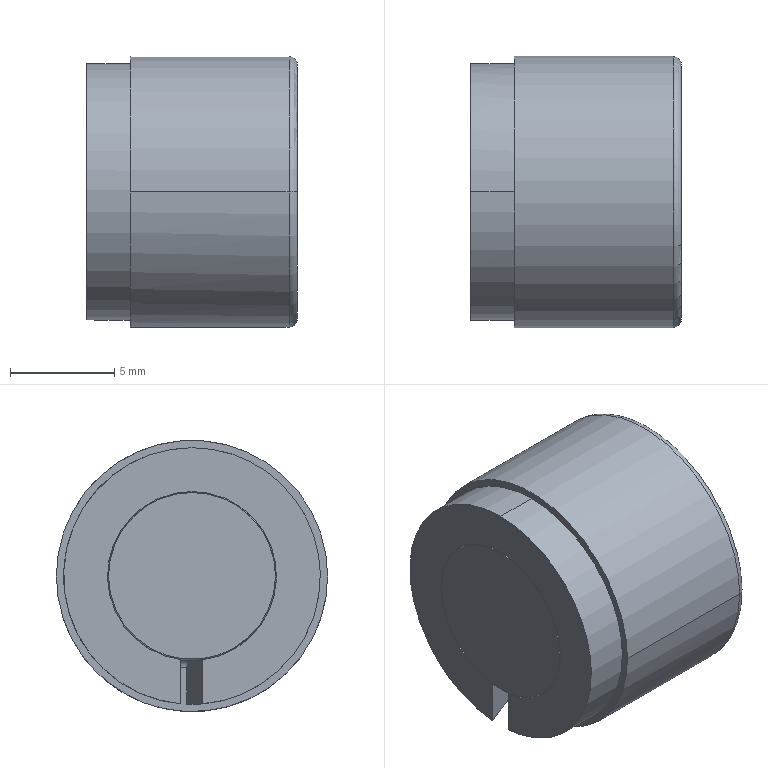Part | STEP file | Positioning_id1950_x_t | 1 solid | 27 faces | box 10.1 x 13 x 13 mm | volume 1181 mm3 | plane 13 | cylinder 10 | torus 4 | commonest cylinder face diameters 8.1 x3 12.3 x3 8 x2 13 x2